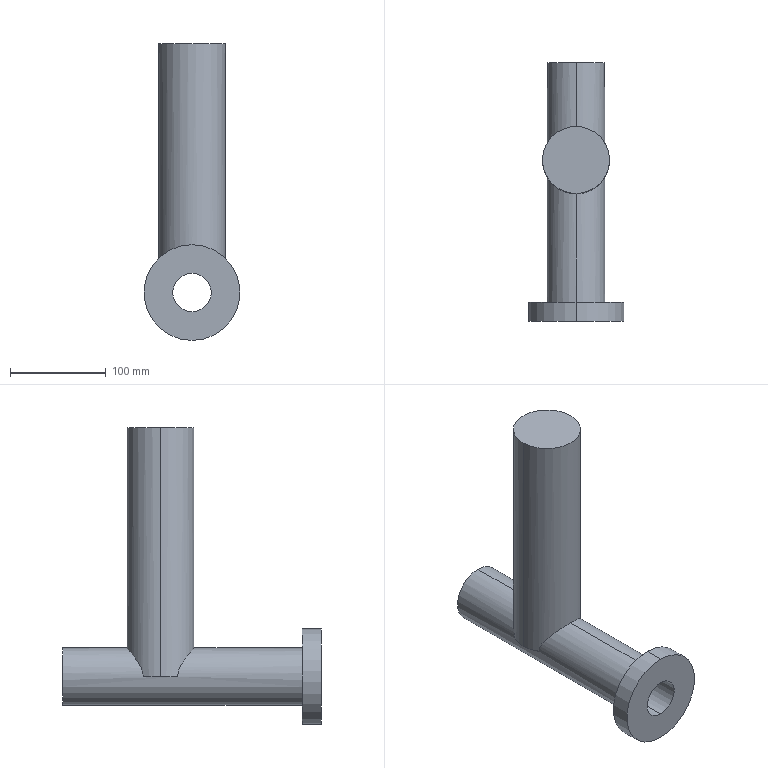Part | SolidWorks | 1 solid | 14 faces | box 100 x 270 x 310 mm | volume 1436503 mm3 | cylinder 8 | plane 6 | commonest cylinder face diameters 40 x2 60 x2 70 x2 100 x2
STEP:
#1=CARTESIAN_POINT('',(0.,-135.,-20.));
#2=VERTEX_POINT('',#1);
#3=CARTESIAN_POINT('',(0.,-135.,20.));
#4=VERTEX_POINT('',#3);
#5=CARTESIAN_POINT('',(0.,-135.,0.));
#6=DIRECTION('',(0.,1.,0.));
#7=DIRECTION('',(0.,0.,1.));
#8=AXIS2_PLACEMENT_3D('',#5,#6,#7);
#9=CIRCLE('',#8,20.);
#10=EDGE_CURVE('',#2,#4,#9,.T.);
#11=ORIENTED_EDGE('',*,*,#10,.F.);
#12=CARTESIAN_POINT('',(0.,135.,-20.));
#13=VERTEX_POINT('',#12);
#14=CARTESIAN_POINT('',(0.,-156.,-20.));
#15=DIRECTION('',(0.,1.,0.));
#16=VECTOR('',#15,1000.);
#17=LINE('',#14,#16);
#18=EDGE_CURVE('',#2,#13,#17,.T.);
#19=ORIENTED_EDGE('',*,*,#18,.T.);
#20=CARTESIAN_POINT('',(0.,135.,20.));
#21=VERTEX_POINT('',#20);
#22=CARTESIAN_POINT('',(0.,135.,0.));
#23=DIRECTION('',(0.,1.,0.));
#24=DIRECTION('',(0.,0.,1.));
#25=AXIS2_PLACEMENT_3D('',#22,#23,#24);
#26=CIRCLE('',#25,20.);
#27=EDGE_CURVE('',#13,#21,#26,.T.);
#28=ORIENTED_EDGE('',*,*,#27,.T.);
#29=CARTESIAN_POINT('',(0.,-156.,20.));
#30=DIRECTION('',(0.,1.,0.));
#31=VECTOR('',#30,1000.);
#32=LINE('',#29,#31);
#33=EDGE_CURVE('',#4,#21,#32,.T.);
#34=ORIENTED_EDGE('',*,*,#33,.F.);
#35=EDGE_LOOP('',(#11,#19,#28,#34));
#36=FACE_OUTER_BOUND('',#35,.T.);
#37=CARTESIAN_POINT('',(0.,-156.,0.));
#38=DIRECTION('',(0.,1.,0.));
#39=DIRECTION('',(0.,0.,1.));
#40=AXIS2_PLACEMENT_3D('',#37,#38,#39);
#41=CYLINDRICAL_SURFACE('',#40,20.);
#42=ADVANCED_FACE('',(#36),#41,.F.);
#43=CARTESIAN_POINT('',(35.,32.949,260.));
#44=VERTEX_POINT('',#43);
#45=CARTESIAN_POINT('',(-35.,32.949,260.));
#46=VERTEX_POINT('',#45);
#47=CARTESIAN_POINT('',(0.,32.949,260.));
#48=DIRECTION('',(0.,0.,1.));
#49=DIRECTION('',(1.,0.,0.));
#50=AXIS2_PLACEMENT_3D('',#47,#48,#49);
#51=CIRCLE('',#50,35.);
#52=EDGE_CURVE('',#44,#46,#51,.T.);
#53=ORIENTED_EDGE('',*,*,#52,.F.);
#54=CARTESIAN_POINT('',(35.,32.949,0.));
#55=VERTEX_POINT('',#54);
#56=CARTESIAN_POINT('',(35.,32.949,260.));
#57=DIRECTION('',(0.,0.,-1.));
#58=VECTOR('',#57,1000.);
#59=LINE('',#56,#58);
#60=EDGE_CURVE('',#44,#55,#59,.T.);
#61=ORIENTED_EDGE('',*,*,#60,.T.);
#62=CARTESIAN_POINT('',(30.,50.977,0.));
#63=VERTEX_POINT('',#62);
#64=CARTESIAN_POINT('',(0.,32.949,0.));
#65=DIRECTION('',(0.,0.,1.));
#66=DIRECTION('',(1.,0.,0.));
#67=AXIS2_PLACEMENT_3D('',#64,#65,#66);
#68=CIRCLE('',#67,35.);
#69=EDGE_CURVE('',#55,#63,#68,.T.);
#70=ORIENTED_EDGE('',*,*,#69,.T.);
#71=CARTESIAN_POINT('',(0.,67.949,30.));
#72=VERTEX_POINT('',#71);
#73=CARTESIAN_POINT('',(30.,50.977,0.));
#74=CARTESIAN_POINT('',(30.,50.977,1.072));
#75=CARTESIAN_POINT('',(29.943,51.073,2.123));
#76=CARTESIAN_POINT('',(29.779,51.34,3.672));
#77=CARTESIAN_POINT('',(29.711,51.449,4.183));
#78=CARTESIAN_POINT('',(29.551,51.705,5.198));
#79=CARTESIAN_POINT('',(29.457,51.852,5.703));
#80=CARTESIAN_POINT('',(29.142,52.337,7.194));
#81=CARTESIAN_POINT('',(28.889,52.715,8.148));
#82=CARTESIAN_POINT('',(28.303,53.545,9.994));
#83=CARTESIAN_POINT('',(27.971,53.996,10.886));
#84=CARTESIAN_POINT('',(27.231,54.945,12.624));
#85=CARTESIAN_POINT('',(26.821,55.446,13.472));
#86=CARTESIAN_POINT('',(25.936,56.46,15.106));
#87=CARTESIAN_POINT('',(25.461,56.975,15.892));
#88=CARTESIAN_POINT('',(23.938,58.523,18.174));
#89=CARTESIAN_POINT('',(22.793,59.56,19.593));
#90=CARTESIAN_POINT('',(21.178,60.817,21.253));
#91=CARTESIAN_POINT('',(20.846,61.067,21.579));
#92=CARTESIAN_POINT('',(20.162,61.562,22.22));
#93=CARTESIAN_POINT('',(19.809,61.807,22.535));
#94=CARTESIAN_POINT('',(18.729,62.529,23.454));
#95=CARTESIAN_POINT('',(17.979,62.992,24.035));
#96=CARTESIAN_POINT('',(15.631,64.316,25.677));
#97=CARTESIAN_POINT('',(13.938,65.114,26.642));
#98=CARTESIAN_POINT('',(10.239,66.476,28.271));
#99=CARTESIAN_POINT('',(8.301,67.013,28.904));
#100=CARTESIAN_POINT('',(5.758,67.476,29.447));
#101=CARTESIAN_POINT('',(5.244,67.558,29.543));
#102=CARTESIAN_POINT('',(4.201,67.7,29.709));
#103=CARTESIAN_POINT('',(3.675,67.76,29.779));
#104=CARTESIAN_POINT('',(2.1,67.902,29.945));
#105=CARTESIAN_POINT('',(1.05,67.949,30.));
#106=CARTESIAN_POINT('',(0.,67.949,30.));
#107=B_SPLINE_CURVE_WITH_KNOTS('',3,(#73,#74,#75,#76,#77,#78,#79,#80,#81,#82,#83,#84,#85,#86,#87,#88,#89,#90,#91,#92,#93,#94,#95,#96,#97,#98,#99,#100,#101,#102,#103,#104,#105,#106),.UNSPECIFIED.,.F.,.F.,(4,2,2,2,2,2,2,2,2,2,2,2,2,2,2,2,4),(0.,0.00316,0.00474,0.00632,0.00948,0.01264,0.0158,0.01896,0.02528,0.02686,0.02844,0.0316,0.03792,0.04424,0.04582,0.0474,0.05056),.UNSPECIFIED.);
#108=EDGE_CURVE('',#63,#72,#107,.T.);
#109=ORIENTED_EDGE('',*,*,#108,.T.);
#110=CARTESIAN_POINT('',(-30.,50.977,0.));
#111=VERTEX_POINT('',#110);
#112=CARTESIAN_POINT('',(0.,67.949,30.));
#113=CARTESIAN_POINT('',(-1.049,67.949,30.));
#114=CARTESIAN_POINT('',(-2.098,67.902,29.945));
#115=CARTESIAN_POINT('',(-3.672,67.76,29.779));
#116=CARTESIAN_POINT('',(-4.199,67.7,29.709));
#117=CARTESIAN_POINT('',(-5.238,67.559,29.544));
#118=CARTESIAN_POINT('',(-5.751,67.477,29.448));
#119=CARTESIAN_POINT('',(-7.274,67.2,29.123));
#120=CARTESIAN_POINT('',(-8.267,66.974,28.856));
#121=CARTESIAN_POINT('',(-9.724,66.575,28.385));
#122=CARTESIAN_POINT('',(-10.205,66.432,28.216));
#123=CARTESIAN_POINT('',(-11.155,66.128,27.854));
#124=CARTESIAN_POINT('',(-11.625,65.966,27.661));
#125=CARTESIAN_POINT('',(-13.924,65.12,26.649));
#126=CARTESIAN_POINT('',(-15.621,64.322,25.684));
#127=CARTESIAN_POINT('',(-17.591,63.211,24.306));
#128=CARTESIAN_POINT('',(-17.978,62.982,24.021));
#129=CARTESIAN_POINT('',(-18.732,62.518,23.438));
#130=CARTESIAN_POINT('',(-19.099,62.282,23.14));
#131=CARTESIAN_POINT('',(-20.172,61.564,22.225));
#132=CARTESIAN_POINT('',(-20.849,61.073,21.591));
#133=CARTESIAN_POINT('',(-22.778,59.573,19.611));
#134=CARTESIAN_POINT('',(-23.926,58.536,18.192));
#135=CARTESIAN_POINT('',(-25.205,57.236,16.277));
#136=CARTESIAN_POINT('',(-25.453,56.975,15.885));
#137=CARTESIAN_POINT('',(-25.931,56.459,15.093));
#138=CARTESIAN_POINT('',(-26.16,56.203,14.692));
#139=CARTESIAN_POINT('',(-26.822,55.444,13.47));
#140=CARTESIAN_POINT('',(-27.226,54.951,12.634));
#141=CARTESIAN_POINT('',(-27.963,54.006,10.906));
#142=CARTESIAN_POINT('',(-28.296,53.555,10.014));
#143=CARTESIAN_POINT('',(-28.885,52.721,8.161));
#144=CARTESIAN_POINT('',(-29.142,52.337,7.195));
#145=CARTESIAN_POINT('',(-29.559,51.696,5.225));
#146=CARTESIAN_POINT('',(-29.721,51.435,4.216));
#147=CARTESIAN_POINT('',(-29.886,51.165,2.659));
#148=CARTESIAN_POINT('',(-29.929,51.095,2.131));
#149=CARTESIAN_POINT('',(-29.986,51.001,1.068));
#150=CARTESIAN_POINT('',(-30.,50.977,0.5349));
#151=CARTESIAN_POINT('',(-30.,50.977,0.));
#152=B_SPLINE_CURVE_WITH_KNOTS('',3,(#112,#113,#114,#115,#116,#117,#118,#119,#120,#121,#122,#123,#124,#125,#126,#127,#128,#129,#130,#131,#132,#133,#134,#135,#136,#137,#138,#139,#140,#141,#142,#143,#144,#145,#146,#147,#148,#149,#150,#151),.UNSPECIFIED.,.F.,.F.,(4,2,2,2,2,2,2,2,2,2,2,2,2,2,2,2,2,2,2,4),(0.05056,0.05372,0.05529,0.05687,0.06003,0.0616,0.06318,0.06949,0.07107,0.07264,0.0758,0.08211,0.08368,0.08526,0.08842,0.09157,0.09473,0.09788,0.09946,0.101),.UNSPECIFIED.);
#153=EDGE_CURVE('',#72,#111,#152,.T.);
#154=ORIENTED_EDGE('',*,*,#153,.T.);
#155=CARTESIAN_POINT('',(-35.,32.949,0.));
#156=VERTEX_POINT('',#155);
#157=CARTESIAN_POINT('',(0.,32.949,0.));
#158=DIRECTION('',(0.,0.,1.));
#159=DIRECTION('',(1.,0.,0.));
#160=AXIS2_PLACEMENT_3D('',#157,#158,#159);
#161=CIRCLE('',#160,35.);
#162=EDGE_CURVE('',#111,#156,#161,.T.);
#163=ORIENTED_EDGE('',*,*,#162,.T.);
#164=CARTESIAN_POINT('',(-35.,32.949,260.));
#165=DIRECTION('',(0.,0.,-1.));
#166=VECTOR('',#165,1000.);
#167=LINE('',#164,#166);
#168=EDGE_CURVE('',#46,#156,#167,.T.);
#169=ORIENTED_EDGE('',*,*,#168,.F.);
#170=EDGE_LOOP('',(#53,#61,#70,#109,#154,#163,#169));
#171=FACE_OUTER_BOUND('',#170,.T.);
#172=CARTESIAN_POINT('',(0.,32.949,260.));
#173=DIRECTION('',(0.,0.,-1.));
#174=DIRECTION('',(-1.,0.,0.));
#175=AXIS2_PLACEMENT_3D('',#172,#173,#174);
#176=CYLINDRICAL_SURFACE('',#175,35.);
#177=ADVANCED_FACE('',(#171),#176,.T.);
#178=CARTESIAN_POINT('',(0.,-135.,50.));
#179=VERTEX_POINT('',#178);
#180=CARTESIAN_POINT('',(0.,-135.,-50.));
#181=VERTEX_POINT('',#180);
#182=CARTESIAN_POINT('',(0.,-135.,0.));
#183=DIRECTION('',(0.,1.,0.));
#184=DIRECTION('',(0.,0.,1.));
#185=AXIS2_PLACEMENT_3D('',#182,#183,#184);
#186=CIRCLE('',#185,50.);
#187=EDGE_CURVE('',#179,#181,#186,.T.);
#188=ORIENTED_EDGE('',*,*,#187,.T.);
#189=CARTESIAN_POINT('',(0.,-115.,-50.));
#190=VERTEX_POINT('',#189);
#191=CARTESIAN_POINT('',(0.,135.,-50.));
#192=DIRECTION('',(0.,1.,0.));
#193=VECTOR('',#192,1000.);
#194=LINE('',#191,#193);
#195=EDGE_CURVE('',#181,#190,#194,.T.);
#196=ORIENTED_EDGE('',*,*,#195,.T.);
#197=CARTESIAN_POINT('',(0.,-115.,50.));
#198=VERTEX_POINT('',#197);
#199=CARTESIAN_POINT('',(0.,-115.,0.));
#200=DIRECTION('',(0.,1.,0.));
#201=DIRECTION('',(0.,0.,1.));
#202=AXIS2_PLACEMENT_3D('',#199,#200,#201);
#203=CIRCLE('',#202,50.);
#204=EDGE_CURVE('',#198,#190,#203,.T.);
#205=ORIENTED_EDGE('',*,*,#204,.F.);
#206=CARTESIAN_POINT('',(0.,135.,50.));
#207=DIRECTION('',(0.,1.,0.));
#208=VECTOR('',#207,1000.);
#209=LINE('',#206,#208);
#210=EDGE_CURVE('',#179,#198,#209,.T.);
#211=ORIENTED_EDGE('',*,*,#210,.F.);
#212=EDGE_LOOP('',(#188,#196,#205,#211));
#213=FACE_OUTER_BOUND('',#212,.T.);
#214=CARTESIAN_POINT('',(0.,135.,0.));
#215=DIRECTION('',(0.,1.,0.));
#216=DIRECTION('',(0.,0.,1.));
#217=AXIS2_PLACEMENT_3D('',#214,#215,#216);
#218=CYLINDRICAL_SURFACE('',#217,50.);
#219=ADVANCED_FACE('',(#213),#218,.T.);
#220=CARTESIAN_POINT('',(0.,-115.,30.));
#221=VERTEX_POINT('',#220);
#222=CARTESIAN_POINT('',(0.,-115.,-30.));
#223=VERTEX_POINT('',#222);
#224=CARTESIAN_POINT('',(0.,-115.,0.));
#225=DIRECTION('',(0.,1.,0.));
#226=DIRECTION('',(0.,0.,1.));
#227=AXIS2_PLACEMENT_3D('',#224,#225,#226);
#228=CIRCLE('',#227,30.);
#229=EDGE_CURVE('',#221,#223,#228,.T.);
#230=ORIENTED_EDGE('',*,*,#229,.T.);
#231=CARTESIAN_POINT('',(0.,135.,-30.));
#232=VERTEX_POINT('',#231);
#233=CARTESIAN_POINT('',(0.,135.,-30.));
#234=DIRECTION('',(0.,1.,0.));
#235=VECTOR('',#234,1000.);
#236=LINE('',#233,#235);
#237=EDGE_CURVE('',#223,#232,#236,.T.);
#238=ORIENTED_EDGE('',*,*,#237,.T.);
#239=CARTESIAN_POINT('',(0.,135.,30.));
#240=VERTEX_POINT('',#239);
#241=CARTESIAN_POINT('',(0.,135.,0.));
#242=DIRECTION('',(0.,1.,0.));
#243=DIRECTION('',(0.,0.,1.));
#244=AXIS2_PLACEMENT_3D('',#241,#242,#243);
#245=CIRCLE('',#244,30.);
#246=EDGE_CURVE('',#240,#232,#245,.T.);
#247=ORIENTED_EDGE('',*,*,#246,.F.);
#248=CARTESIAN_POINT('',(0.,135.,30.));
#249=DIRECTION('',(0.,1.,0.));
#250=VECTOR('',#249,1000.);
#251=LINE('',#248,#250);
#252=EDGE_CURVE('',#72,#240,#251,.T.);
#253=ORIENTED_EDGE('',*,*,#252,.F.);
#254=ORIENTED_EDGE('',*,*,#108,.F.);
#255=CARTESIAN_POINT('',(30.,14.921,0.));
#256=VERTEX_POINT('',#255);
#257=CARTESIAN_POINT('',(30.,135.,0.));
#258=DIRECTION('',(0.,1.,0.));
#259=VECTOR('',#258,1000.);
#260=LINE('',#257,#259);
#261=EDGE_CURVE('',#256,#63,#260,.T.);
#262=ORIENTED_EDGE('',*,*,#261,.F.);
#263=CARTESIAN_POINT('',(0.,-2.051,30.));
#264=VERTEX_POINT('',#263);
#265=CARTESIAN_POINT('',(0.,-2.051,30.));
#266=CARTESIAN_POINT('',(1.049,-2.051,30.));
#267=CARTESIAN_POINT('',(2.098,-2.004,29.945));
#268=CARTESIAN_POINT('',(3.672,-1.862,29.779));
#269=CARTESIAN_POINT('',(4.199,-1.802,29.709));
#270=CARTESIAN_POINT('',(5.238,-1.661,29.544));
#271=CARTESIAN_POINT('',(5.751,-1.579,29.448));
#272=CARTESIAN_POINT('',(7.274,-1.302,29.123));
#273=CARTESIAN_POINT('',(8.267,-1.075,28.856));
#274=CARTESIAN_POINT('',(9.724,-0.6767,28.385));
#275=CARTESIAN_POINT('',(10.205,-0.534,28.216));
#276=CARTESIAN_POINT('',(11.155,-0.2296,27.854));
#277=CARTESIAN_POINT('',(11.625,-0.06767,27.661));
#278=CARTESIAN_POINT('',(13.924,0.7783,26.649));
#279=CARTESIAN_POINT('',(15.621,1.576,25.684));
#280=CARTESIAN_POINT('',(17.591,2.687,24.306));
#281=CARTESIAN_POINT('',(17.978,2.916,24.021));
#282=CARTESIAN_POINT('',(18.732,3.38,23.438));
#283=CARTESIAN_POINT('',(19.099,3.616,23.14));
#284=CARTESIAN_POINT('',(20.172,4.334,22.225));
#285=CARTESIAN_POINT('',(20.849,4.825,21.591));
#286=CARTESIAN_POINT('',(22.778,6.325,19.611));
#287=CARTESIAN_POINT('',(23.926,7.362,18.192));
#288=CARTESIAN_POINT('',(25.205,8.662,16.277));
#289=CARTESIAN_POINT('',(25.453,8.923,15.885));
#290=CARTESIAN_POINT('',(25.931,9.439,15.093));
#291=CARTESIAN_POINT('',(26.16,9.695,14.692));
#292=CARTESIAN_POINT('',(26.822,10.454,13.47));
#293=CARTESIAN_POINT('',(27.226,10.947,12.634));
#294=CARTESIAN_POINT('',(27.963,11.892,10.906));
#295=CARTESIAN_POINT('',(28.296,12.343,10.014));
#296=CARTESIAN_POINT('',(28.885,13.177,8.161));
#297=CARTESIAN_POINT('',(29.142,13.561,7.195));
#298=CARTESIAN_POINT('',(29.559,14.203,5.225));
#299=CARTESIAN_POINT('',(29.721,14.463,4.216));
#300=CARTESIAN_POINT('',(29.886,14.733,2.659));
#301=CARTESIAN_POINT('',(29.929,14.804,2.131));
#302=CARTESIAN_POINT('',(29.986,14.897,1.068));
#303=CARTESIAN_POINT('',(30.,14.921,0.5349));
#304=CARTESIAN_POINT('',(30.,14.921,0.));
#305=B_SPLINE_CURVE_WITH_KNOTS('',3,(#265,#266,#267,#268,#269,#270,#271,#272,#273,#274,#275,#276,#277,#278,#279,#280,#281,#282,#283,#284,#285,#286,#287,#288,#289,#290,#291,#292,#293,#294,#295,#296,#297,#298,#299,#300,#301,#302,#303,#304),.UNSPECIFIED.,.F.,.F.,(4,2,2,2,2,2,2,2,2,2,2,2,2,2,2,2,2,2,2,4),(0.05056,0.05372,0.05529,0.05687,0.06003,0.0616,0.06318,0.06949,0.07107,0.07264,0.0758,0.08211,0.08368,0.08526,0.08842,0.09157,0.09473,0.09788,0.09946,0.101),.UNSPECIFIED.);
#306=EDGE_CURVE('',#264,#256,#305,.T.);
#307=ORIENTED_EDGE('',*,*,#306,.F.);
#308=CARTESIAN_POINT('',(0.,135.,30.));
#309=DIRECTION('',(0.,1.,0.));
#310=VECTOR('',#309,1000.);
#311=LINE('',#308,#310);
#312=EDGE_CURVE('',#221,#264,#311,.T.);
#313=ORIENTED_EDGE('',*,*,#312,.F.);
#314=EDGE_LOOP('',(#230,#238,#247,#253,#254,#262,#307,#313));
#315=FACE_OUTER_BOUND('',#314,.T.);
#316=CARTESIAN_POINT('',(0.,135.,0.));
#317=DIRECTION('',(0.,1.,0.));
#318=DIRECTION('',(0.,0.,1.));
#319=AXIS2_PLACEMENT_3D('',#316,#317,#318);
#320=CYLINDRICAL_SURFACE('',#319,30.);
#321=ADVANCED_FACE('',(#315),#320,.T.);
#322=ORIENTED_EDGE('',*,*,#237,.F.);
#323=CARTESIAN_POINT('',(0.,-115.,0.));
#324=DIRECTION('',(0.,1.,0.));
#325=DIRECTION('',(0.,0.,1.));
#326=AXIS2_PLACEMENT_3D('',#323,#324,#325);
#327=CIRCLE('',#326,30.);
#328=EDGE_CURVE('',#223,#221,#327,.T.);
#329=ORIENTED_EDGE('',*,*,#328,.T.);
#330=ORIENTED_EDGE('',*,*,#312,.T.);
#331=CARTESIAN_POINT('',(-30.,14.921,0.));
#332=VERTEX_POINT('',#331);
#333=CARTESIAN_POINT('',(-30.,14.921,0.));
#334=CARTESIAN_POINT('',(-30.,14.921,1.072));
#335=CARTESIAN_POINT('',(-29.943,14.825,2.123));
#336=CARTESIAN_POINT('',(-29.779,14.558,3.672));
#337=CARTESIAN_POINT('',(-29.711,14.449,4.183));
#338=CARTESIAN_POINT('',(-29.551,14.193,5.198));
#339=CARTESIAN_POINT('',(-29.457,14.046,5.703));
#340=CARTESIAN_POINT('',(-29.142,13.561,7.194));
#341=CARTESIAN_POINT('',(-28.889,13.183,8.148));
#342=CARTESIAN_POINT('',(-28.303,12.353,9.994));
#343=CARTESIAN_POINT('',(-27.971,11.902,10.886));
#344=CARTESIAN_POINT('',(-27.231,10.953,12.624));
#345=CARTESIAN_POINT('',(-26.821,10.453,13.472));
#346=CARTESIAN_POINT('',(-25.936,9.438,15.106));
#347=CARTESIAN_POINT('',(-25.461,8.923,15.892));
#348=CARTESIAN_POINT('',(-23.938,7.375,18.174));
#349=CARTESIAN_POINT('',(-22.793,6.338,19.593));
#350=CARTESIAN_POINT('',(-21.178,5.081,21.253));
#351=CARTESIAN_POINT('',(-20.846,4.831,21.579));
#352=CARTESIAN_POINT('',(-20.162,4.336,22.22));
#353=CARTESIAN_POINT('',(-19.809,4.091,22.535));
#354=CARTESIAN_POINT('',(-18.729,3.369,23.454));
#355=CARTESIAN_POINT('',(-17.979,2.906,24.035));
#356=CARTESIAN_POINT('',(-15.631,1.582,25.677));
#357=CARTESIAN_POINT('',(-13.938,0.7838,26.642));
#358=CARTESIAN_POINT('',(-10.239,-0.5779,28.271));
#359=CARTESIAN_POINT('',(-8.301,-1.115,28.904));
#360=CARTESIAN_POINT('',(-5.758,-1.578,29.447));
#361=CARTESIAN_POINT('',(-5.244,-1.66,29.543));
#362=CARTESIAN_POINT('',(-4.201,-1.802,29.709));
#363=CARTESIAN_POINT('',(-3.675,-1.862,29.779));
#364=CARTESIAN_POINT('',(-2.1,-2.004,29.945));
#365=CARTESIAN_POINT('',(-1.05,-2.051,30.));
#366=CARTESIAN_POINT('',(0.,-2.051,30.));
#367=B_SPLINE_CURVE_WITH_KNOTS('',3,(#333,#334,#335,#336,#337,#338,#339,#340,#341,#342,#343,#344,#345,#346,#347,#348,#349,#350,#351,#352,#353,#354,#355,#356,#357,#358,#359,#360,#361,#362,#363,#364,#365,#366),.UNSPECIFIED.,.F.,.F.,(4,2,2,2,2,2,2,2,2,2,2,2,2,2,2,2,4),(0.,0.00316,0.00474,0.00632,0.00948,0.01264,0.0158,0.01896,0.02528,0.02686,0.02844,0.0316,0.03792,0.04424,0.04582,0.0474,0.05056),.UNSPECIFIED.);
#368=EDGE_CURVE('',#332,#264,#367,.T.);
#369=ORIENTED_EDGE('',*,*,#368,.F.);
#370=CARTESIAN_POINT('',(-30.,135.,0.));
#371=DIRECTION('',(0.,-1.,0.));
#372=VECTOR('',#371,1000.);
#373=LINE('',#370,#372);
#374=EDGE_CURVE('',#111,#332,#373,.T.);
#375=ORIENTED_EDGE('',*,*,#374,.F.);
#376=ORIENTED_EDGE('',*,*,#153,.F.);
#377=ORIENTED_EDGE('',*,*,#252,.T.);
#378=CARTESIAN_POINT('',(0.,135.,0.));
#379=DIRECTION('',(0.,1.,0.));
#380=DIRECTION('',(0.,0.,1.));
#381=AXIS2_PLACEMENT_3D('',#378,#379,#380);
#382=CIRCLE('',#381,30.);
#383=EDGE_CURVE('',#232,#240,#382,.T.);
#384=ORIENTED_EDGE('',*,*,#383,.F.);
#385=EDGE_LOOP('',(#322,#329,#330,#369,#375,#376,#377,#384));
#386=FACE_OUTER_BOUND('',#385,.T.);
#387=CARTESIAN_POINT('',(0.,135.,0.));
#388=DIRECTION('',(0.,1.,0.));
#389=DIRECTION('',(0.,0.,1.));
#390=AXIS2_PLACEMENT_3D('',#387,#388,#389);
#391=CYLINDRICAL_SURFACE('',#390,30.);
#392=ADVANCED_FACE('',(#386),#391,.T.);
#393=CARTESIAN_POINT('',(0.,135.,0.));
#394=DIRECTION('',(0.,1.,0.));
#395=DIRECTION('',(0.,0.,1.));
#396=AXIS2_PLACEMENT_3D('',#393,#394,#395);
#397=CIRCLE('',#396,20.);
#398=EDGE_CURVE('',#21,#13,#397,.T.);
#399=ORIENTED_EDGE('',*,*,#398,.F.);
#400=ORIENTED_EDGE('',*,*,#27,.F.);
#401=EDGE_LOOP('',(#399,#400));
#402=FACE_BOUND('',#401,.T.);
#403=ORIENTED_EDGE('',*,*,#246,.T.);
#404=ORIENTED_EDGE('',*,*,#383,.T.);
#405=EDGE_LOOP('',(#403,#404));
#406=FACE_OUTER_BOUND('',#405,.T.);
#407=CARTESIAN_POINT('',(30.,135.,0.));
#408=DIRECTION('',(0.,-1.,0.));
#409=DIRECTION('',(0.,0.,-1.));
#410=AXIS2_PLACEMENT_3D('',#407,#408,#409);
#411=PLANE('',#410);
#412=ADVANCED_FACE('',(#402,#406),#411,.F.);
#413=CARTESIAN_POINT('',(0.,-135.,0.));
#414=DIRECTION('',(0.,1.,0.));
#415=DIRECTION('',(0.,0.,1.));
#416=AXIS2_PLACEMENT_3D('',#413,#414,#415);
#417=CIRCLE('',#416,20.);
#418=EDGE_CURVE('',#4,#2,#417,.T.);
#419=ORIENTED_EDGE('',*,*,#418,.T.);
#420=ORIENTED_EDGE('',*,*,#10,.T.);
#421=EDGE_LOOP('',(#419,#420));
#422=FACE_BOUND('',#421,.T.);
#423=ORIENTED_EDGE('',*,*,#187,.F.);
#424=CARTESIAN_POINT('',(0.,-135.,0.));
#425=DIRECTION('',(0.,1.,0.));
#426=DIRECTION('',(0.,0.,1.));
#427=AXIS2_PLACEMENT_3D('',#424,#425,#426);
#428=CIRCLE('',#427,50.);
#429=EDGE_CURVE('',#181,#179,#428,.T.);
#430=ORIENTED_EDGE('',*,*,#429,.F.);
#431=EDGE_LOOP('',(#423,#430));
#432=FACE_OUTER_BOUND('',#431,.T.);
#433=CARTESIAN_POINT('',(0.,-135.,0.));
#434=DIRECTION('',(0.,1.,0.));
#435=DIRECTION('',(0.,0.,1.));
#436=AXIS2_PLACEMENT_3D('',#433,#434,#435);
#437=PLANE('',#436);
#438=ADVANCED_FACE('',(#422,#432),#437,.F.);
#439=ORIENTED_EDGE('',*,*,#195,.F.);
#440=ORIENTED_EDGE('',*,*,#429,.T.);
#441=ORIENTED_EDGE('',*,*,#210,.T.);
#442=CARTESIAN_POINT('',(0.,-115.,0.));
#443=DIRECTION('',(0.,1.,0.));
#444=DIRECTION('',(0.,0.,1.));
#445=AXIS2_PLACEMENT_3D('',#442,#443,#444);
#446=CIRCLE('',#445,50.);
#447=EDGE_CURVE('',#190,#198,#446,.T.);
#448=ORIENTED_EDGE('',*,*,#447,.F.);
#449=EDGE_LOOP('',(#439,#440,#441,#448));
#450=FACE_OUTER_BOUND('',#449,.T.);
#451=CARTESIAN_POINT('',(0.,135.,0.));
#452=DIRECTION('',(0.,1.,0.));
#453=DIRECTION('',(0.,0.,1.));
#454=AXIS2_PLACEMENT_3D('',#451,#452,#453);
#455=CYLINDRICAL_SURFACE('',#454,50.);
#456=ADVANCED_FACE('',(#450),#455,.T.);
#457=ORIENTED_EDGE('',*,*,#229,.F.);
#458=ORIENTED_EDGE('',*,*,#328,.F.);
#459=EDGE_LOOP('',(#457,#458));
#460=FACE_BOUND('',#459,.T.);
#461=ORIENTED_EDGE('',*,*,#204,.T.);
#462=ORIENTED_EDGE('',*,*,#447,.T.);
#463=EDGE_LOOP('',(#461,#462));
#464=FACE_OUTER_BOUND('',#463,.T.);
#465=CARTESIAN_POINT('',(50.,-115.,0.));
#466=DIRECTION('',(0.,-1.,0.));
#467=DIRECTION('',(0.,0.,-1.));
#468=AXIS2_PLACEMENT_3D('',#465,#466,#467);
#469=PLANE('',#468);
#470=ADVANCED_FACE('',(#460,#464),#469,.F.);
#471=ORIENTED_EDGE('',*,*,#60,.F.);
#472=CARTESIAN_POINT('',(0.,32.949,260.));
#473=DIRECTION('',(0.,0.,1.));
#474=DIRECTION('',(1.,0.,0.));
#475=AXIS2_PLACEMENT_3D('',#472,#473,#474);
#476=CIRCLE('',#475,35.);
#477=EDGE_CURVE('',#46,#44,#476,.T.);
#478=ORIENTED_EDGE('',*,*,#477,.F.);
#479=ORIENTED_EDGE('',*,*,#168,.T.);
#480=CARTESIAN_POINT('',(0.,32.949,0.));
#481=DIRECTION('',(0.,0.,1.));
#482=DIRECTION('',(1.,0.,0.));
#483=AXIS2_PLACEMENT_3D('',#480,#481,#482);
#484=CIRCLE('',#483,35.);
#485=EDGE_CURVE('',#156,#332,#484,.T.);
#486=ORIENTED_EDGE('',*,*,#485,.T.);
#487=ORIENTED_EDGE('',*,*,#368,.T.);
#488=ORIENTED_EDGE('',*,*,#306,.T.);
#489=CARTESIAN_POINT('',(0.,32.949,0.));
#490=DIRECTION('',(0.,0.,1.));
#491=DIRECTION('',(1.,0.,0.));
#492=AXIS2_PLACEMENT_3D('',#489,#490,#491);
#493=CIRCLE('',#492,35.);
#494=EDGE_CURVE('',#256,#55,#493,.T.);
#495=ORIENTED_EDGE('',*,*,#494,.T.);
#496=EDGE_LOOP('',(#471,#478,#479,#486,#487,#488,#495));
#497=FACE_OUTER_BOUND('',#496,.T.);
#498=CARTESIAN_POINT('',(0.,32.949,260.));
#499=DIRECTION('',(0.,0.,-1.));
#500=DIRECTION('',(-1.,0.,0.));
#501=AXIS2_PLACEMENT_3D('',#498,#499,#500);
#502=CYLINDRICAL_SURFACE('',#501,35.);
#503=ADVANCED_FACE('',(#497),#502,.T.);
#504=ORIENTED_EDGE('',*,*,#494,.F.);
#505=ORIENTED_EDGE('',*,*,#261,.T.);
#506=ORIENTED_EDGE('',*,*,#69,.F.);
#507=EDGE_LOOP('',(#504,#505,#506));
#508=FACE_OUTER_BOUND('',#507,.T.);
#509=CARTESIAN_POINT('',(0.,32.949,0.));
#510=DIRECTION('',(0.,0.,1.));
#511=DIRECTION('',(1.,0.,0.));
#512=AXIS2_PLACEMENT_3D('',#509,#510,#511);
#513=PLANE('',#512);
#514=ADVANCED_FACE('',(#508),#513,.F.);
#515=ORIENTED_EDGE('',*,*,#162,.F.);
#516=ORIENTED_EDGE('',*,*,#374,.T.);
#517=ORIENTED_EDGE('',*,*,#485,.F.);
#518=EDGE_LOOP('',(#515,#516,#517));
#519=FACE_OUTER_BOUND('',#518,.T.);
#520=CARTESIAN_POINT('',(0.,32.949,0.));
#521=DIRECTION('',(0.,0.,1.));
#522=DIRECTION('',(1.,0.,0.));
#523=AXIS2_PLACEMENT_3D('',#520,#521,#522);
#524=PLANE('',#523);
#525=ADVANCED_FACE('',(#519),#524,.F.);
#526=ORIENTED_EDGE('',*,*,#477,.T.);
#527=ORIENTED_EDGE('',*,*,#52,.T.);
#528=EDGE_LOOP('',(#526,#527));
#529=FACE_OUTER_BOUND('',#528,.T.);
#530=CARTESIAN_POINT('',(0.,32.949,260.));
#531=DIRECTION('',(0.,0.,1.));
#532=DIRECTION('',(1.,0.,0.));
#533=AXIS2_PLACEMENT_3D('',#530,#531,#532);
#534=PLANE('',#533);
#535=ADVANCED_FACE('',(#529),#534,.T.);
#536=ORIENTED_EDGE('',*,*,#18,.F.);
#537=ORIENTED_EDGE('',*,*,#418,.F.);
#538=ORIENTED_EDGE('',*,*,#33,.T.);
#539=ORIENTED_EDGE('',*,*,#398,.T.);
#540=EDGE_LOOP('',(#536,#537,#538,#539));
#541=FACE_OUTER_BOUND('',#540,.T.);
#542=CARTESIAN_POINT('',(0.,-156.,0.));
#543=DIRECTION('',(0.,1.,0.));
#544=DIRECTION('',(0.,0.,1.));
#545=AXIS2_PLACEMENT_3D('',#542,#543,#544);
#546=CYLINDRICAL_SURFACE('',#545,20.);
#547=ADVANCED_FACE('',(#541),#546,.F.);
#548=CLOSED_SHELL('',(#42,#177,#219,#321,#392,#412,#438,#456,#470,#503,#514,#525,#535,#547));
#549=MANIFOLD_SOLID_BREP('',#548);
#550=CARTESIAN_POINT('',(0.,0.,0.));
#551=DIRECTION('',(0.,0.,1.));
#552=DIRECTION('',(1.,0.,0.));
#553=AXIS2_PLACEMENT_3D('',#550,#551,#552);
#554=(LENGTH_UNIT()NAMED_UNIT(*)SI_UNIT(.MILLI.,.METRE.));
#555=UNCERTAINTY_MEASURE_WITH_UNIT(LENGTH_MEASURE(0.00001),#554,'','');
#556=(NAMED_UNIT(*)PLANE_ANGLE_UNIT()SI_UNIT($,.RADIAN.));
#557=(NAMED_UNIT(*)SI_UNIT($,.STERADIAN.)SOLID_ANGLE_UNIT());
#558=(GEOMETRIC_REPRESENTATION_CONTEXT(3)GLOBAL_UNCERTAINTY_ASSIGNED_CONTEXT((#555))GLOBAL_UNIT_ASSIGNED_CONTEXT((#554,#556,#557))REPRESENTATION_CONTEXT('',''));
#559=ADVANCED_BREP_SHAPE_REPRESENTATION('',(#549,#553),#558);